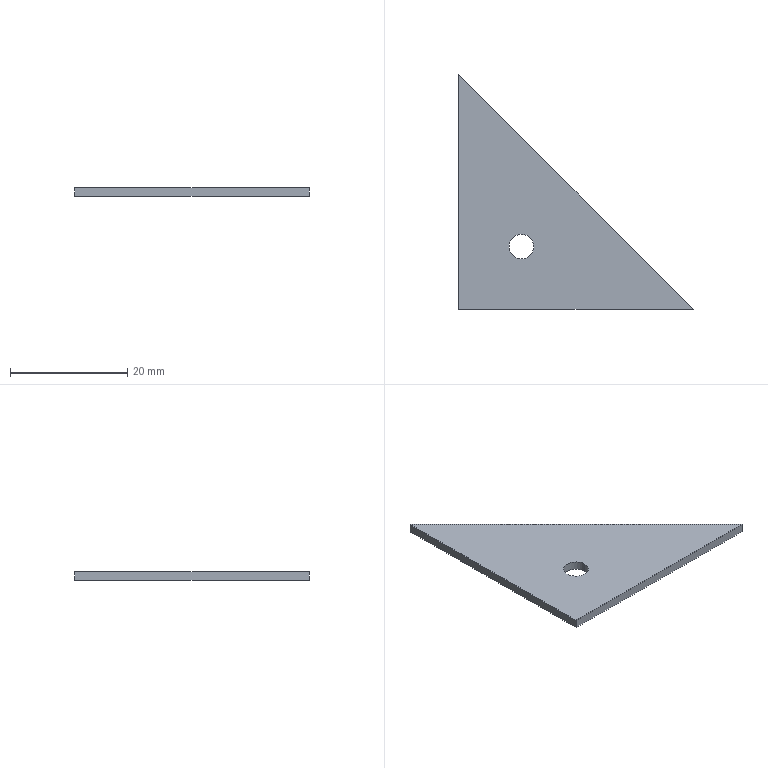Part | SolidWorks | features Cut 1, FlatPattern 1, SMBaseFlange 1, SheetMetal 1 | 1 solid | 7 faces | box 40 x 40 x 1.5 mm | volume 1179 mm3 | plane 5 | cylinder 2 | commonest cylinder face diameters 4.2 x2
STEP:
#1=CARTESIAN_POINT('',(7.968,10.858,-1.5));
#2=VERTEX_POINT('',#1);
#3=CARTESIAN_POINT('',(12.168,10.858,-1.5));
#4=VERTEX_POINT('',#3);
#5=CARTESIAN_POINT('',(10.068,10.858,-1.5));
#6=DIRECTION('',(0.,0.,1.));
#7=DIRECTION('',(1.,0.,0.));
#8=AXIS2_PLACEMENT_3D('',#5,#6,#7);
#9=CIRCLE('',#8,2.1);
#10=EDGE_CURVE('',#2,#4,#9,.T.);
#11=ORIENTED_EDGE('',*,*,#10,.F.);
#12=CARTESIAN_POINT('',(7.968,10.858,0.));
#13=VERTEX_POINT('',#12);
#14=CARTESIAN_POINT('',(7.968,10.858,-1.5));
#15=DIRECTION('',(0.,0.,1.));
#16=VECTOR('',#15,1000.);
#17=LINE('',#14,#16);
#18=EDGE_CURVE('',#2,#13,#17,.T.);
#19=ORIENTED_EDGE('',*,*,#18,.T.);
#20=CARTESIAN_POINT('',(12.168,10.858,0.));
#21=VERTEX_POINT('',#20);
#22=CARTESIAN_POINT('',(10.068,10.858,0.));
#23=DIRECTION('',(0.,0.,1.));
#24=DIRECTION('',(1.,0.,0.));
#25=AXIS2_PLACEMENT_3D('',#22,#23,#24);
#26=CIRCLE('',#25,2.1);
#27=EDGE_CURVE('',#13,#21,#26,.T.);
#28=ORIENTED_EDGE('',*,*,#27,.T.);
#29=CARTESIAN_POINT('',(12.168,10.858,-1.5));
#30=DIRECTION('',(0.,0.,1.));
#31=VECTOR('',#30,1000.);
#32=LINE('',#29,#31);
#33=EDGE_CURVE('',#4,#21,#32,.T.);
#34=ORIENTED_EDGE('',*,*,#33,.F.);
#35=EDGE_LOOP('',(#11,#19,#28,#34));
#36=FACE_OUTER_BOUND('',#35,.T.);
#37=CARTESIAN_POINT('',(10.068,10.858,-1.5));
#38=DIRECTION('',(0.,0.,1.));
#39=DIRECTION('',(1.,0.,0.));
#40=AXIS2_PLACEMENT_3D('',#37,#38,#39);
#41=CYLINDRICAL_SURFACE('',#40,2.1);
#42=ADVANCED_FACE('',(#36),#41,.F.);
#43=CARTESIAN_POINT('',(-0.6321,40.158,0.));
#44=VERTEX_POINT('',#43);
#45=CARTESIAN_POINT('',(-0.6321,0.158,0.));
#46=VERTEX_POINT('',#45);
#47=CARTESIAN_POINT('',(-0.6321,0.158,0.));
#48=DIRECTION('',(0.,-1.,0.));
#49=VECTOR('',#48,1000.);
#50=LINE('',#47,#49);
#51=EDGE_CURVE('',#44,#46,#50,.T.);
#52=ORIENTED_EDGE('',*,*,#51,.F.);
#53=CARTESIAN_POINT('',(-0.6321,40.158,-1.5));
#54=VERTEX_POINT('',#53);
#55=CARTESIAN_POINT('',(-0.6321,40.158,-1.5));
#56=DIRECTION('',(0.,0.,1.));
#57=VECTOR('',#56,1000.);
#58=LINE('',#55,#57);
#59=EDGE_CURVE('',#54,#44,#58,.T.);
#60=ORIENTED_EDGE('',*,*,#59,.F.);
#61=CARTESIAN_POINT('',(-0.6321,0.158,-1.5));
#62=VERTEX_POINT('',#61);
#63=CARTESIAN_POINT('',(-0.6321,0.158,-1.5));
#64=DIRECTION('',(0.,-1.,0.));
#65=VECTOR('',#64,1000.);
#66=LINE('',#63,#65);
#67=EDGE_CURVE('',#54,#62,#66,.T.);
#68=ORIENTED_EDGE('',*,*,#67,.T.);
#69=CARTESIAN_POINT('',(-0.6321,0.158,-1.5));
#70=DIRECTION('',(0.,0.,1.));
#71=VECTOR('',#70,1000.);
#72=LINE('',#69,#71);
#73=EDGE_CURVE('',#62,#46,#72,.T.);
#74=ORIENTED_EDGE('',*,*,#73,.T.);
#75=EDGE_LOOP('',(#52,#60,#68,#74));
#76=FACE_OUTER_BOUND('',#75,.T.);
#77=CARTESIAN_POINT('',(-0.6321,0.158,-1.5));
#78=DIRECTION('',(-1.,0.,0.));
#79=DIRECTION('',(0.,0.,1.));
#80=AXIS2_PLACEMENT_3D('',#77,#78,#79);
#81=PLANE('',#80);
#82=ADVANCED_FACE('',(#76),#81,.T.);
#83=CARTESIAN_POINT('',(39.368,0.158,0.));
#84=VERTEX_POINT('',#83);
#85=CARTESIAN_POINT('',(-0.6321,40.158,0.));
#86=DIRECTION('',(-0.7071,0.7071,0.));
#87=VECTOR('',#86,1000.);
#88=LINE('',#85,#87);
#89=EDGE_CURVE('',#84,#44,#88,.T.);
#90=ORIENTED_EDGE('',*,*,#89,.F.);
#91=CARTESIAN_POINT('',(39.368,0.158,-1.5));
#92=VERTEX_POINT('',#91);
#93=CARTESIAN_POINT('',(39.368,0.158,-1.5));
#94=DIRECTION('',(0.,0.,1.));
#95=VECTOR('',#94,1000.);
#96=LINE('',#93,#95);
#97=EDGE_CURVE('',#92,#84,#96,.T.);
#98=ORIENTED_EDGE('',*,*,#97,.F.);
#99=CARTESIAN_POINT('',(-0.6321,40.158,-1.5));
#100=DIRECTION('',(-0.7071,0.7071,0.));
#101=VECTOR('',#100,1000.);
#102=LINE('',#99,#101);
#103=EDGE_CURVE('',#92,#54,#102,.T.);
#104=ORIENTED_EDGE('',*,*,#103,.T.);
#105=ORIENTED_EDGE('',*,*,#59,.T.);
#106=EDGE_LOOP('',(#90,#98,#104,#105));
#107=FACE_OUTER_BOUND('',#106,.T.);
#108=CARTESIAN_POINT('',(-0.6321,40.158,-1.5));
#109=DIRECTION('',(0.7071,0.7071,0.));
#110=DIRECTION('',(-0.7071,0.7071,0.));
#111=AXIS2_PLACEMENT_3D('',#108,#109,#110);
#112=PLANE('',#111);
#113=ADVANCED_FACE('',(#107),#112,.T.);
#114=CARTESIAN_POINT('',(-0.6321,0.158,0.));
#115=DIRECTION('',(1.,0.,0.));
#116=VECTOR('',#115,1000.);
#117=LINE('',#114,#116);
#118=EDGE_CURVE('',#46,#84,#117,.T.);
#119=ORIENTED_EDGE('',*,*,#118,.F.);
#120=ORIENTED_EDGE('',*,*,#73,.F.);
#121=CARTESIAN_POINT('',(-0.6321,0.158,-1.5));
#122=DIRECTION('',(1.,0.,0.));
#123=VECTOR('',#122,1000.);
#124=LINE('',#121,#123);
#125=EDGE_CURVE('',#62,#92,#124,.T.);
#126=ORIENTED_EDGE('',*,*,#125,.T.);
#127=ORIENTED_EDGE('',*,*,#97,.T.);
#128=EDGE_LOOP('',(#119,#120,#126,#127));
#129=FACE_OUTER_BOUND('',#128,.T.);
#130=CARTESIAN_POINT('',(-0.6321,0.158,-1.5));
#131=DIRECTION('',(0.,-1.,0.));
#132=DIRECTION('',(0.,0.,-1.));
#133=AXIS2_PLACEMENT_3D('',#130,#131,#132);
#134=PLANE('',#133);
#135=ADVANCED_FACE('',(#129),#134,.T.);
#136=CARTESIAN_POINT('',(10.068,10.858,-1.5));
#137=DIRECTION('',(0.,0.,1.));
#138=DIRECTION('',(1.,0.,0.));
#139=AXIS2_PLACEMENT_3D('',#136,#137,#138);
#140=CIRCLE('',#139,2.1);
#141=EDGE_CURVE('',#4,#2,#140,.T.);
#142=ORIENTED_EDGE('',*,*,#141,.T.);
#143=ORIENTED_EDGE('',*,*,#10,.T.);
#144=EDGE_LOOP('',(#142,#143));
#145=FACE_BOUND('',#144,.T.);
#146=ORIENTED_EDGE('',*,*,#67,.F.);
#147=ORIENTED_EDGE('',*,*,#103,.F.);
#148=ORIENTED_EDGE('',*,*,#125,.F.);
#149=EDGE_LOOP('',(#146,#147,#148));
#150=FACE_OUTER_BOUND('',#149,.T.);
#151=CARTESIAN_POINT('',(0.,0.,-1.5));
#152=DIRECTION('',(0.,0.,-1.));
#153=DIRECTION('',(-1.,0.,0.));
#154=AXIS2_PLACEMENT_3D('',#151,#152,#153);
#155=PLANE('',#154);
#156=ADVANCED_FACE('',(#145,#150),#155,.T.);
#157=CARTESIAN_POINT('',(10.068,10.858,0.));
#158=DIRECTION('',(0.,0.,1.));
#159=DIRECTION('',(1.,0.,0.));
#160=AXIS2_PLACEMENT_3D('',#157,#158,#159);
#161=CIRCLE('',#160,2.1);
#162=EDGE_CURVE('',#21,#13,#161,.T.);
#163=ORIENTED_EDGE('',*,*,#162,.F.);
#164=ORIENTED_EDGE('',*,*,#27,.F.);
#165=EDGE_LOOP('',(#163,#164));
#166=FACE_BOUND('',#165,.T.);
#167=ORIENTED_EDGE('',*,*,#51,.T.);
#168=ORIENTED_EDGE('',*,*,#118,.T.);
#169=ORIENTED_EDGE('',*,*,#89,.T.);
#170=EDGE_LOOP('',(#167,#168,#169));
#171=FACE_OUTER_BOUND('',#170,.T.);
#172=CARTESIAN_POINT('',(0.,0.,0.));
#173=DIRECTION('',(0.,0.,-1.));
#174=DIRECTION('',(-1.,0.,0.));
#175=AXIS2_PLACEMENT_3D('',#172,#173,#174);
#176=PLANE('',#175);
#177=ADVANCED_FACE('',(#166,#171),#176,.F.);
#178=ORIENTED_EDGE('',*,*,#18,.F.);
#179=ORIENTED_EDGE('',*,*,#141,.F.);
#180=ORIENTED_EDGE('',*,*,#33,.T.);
#181=ORIENTED_EDGE('',*,*,#162,.T.);
#182=EDGE_LOOP('',(#178,#179,#180,#181));
#183=FACE_OUTER_BOUND('',#182,.T.);
#184=CARTESIAN_POINT('',(10.068,10.858,-1.5));
#185=DIRECTION('',(0.,0.,1.));
#186=DIRECTION('',(1.,0.,0.));
#187=AXIS2_PLACEMENT_3D('',#184,#185,#186);
#188=CYLINDRICAL_SURFACE('',#187,2.1);
#189=ADVANCED_FACE('',(#183),#188,.F.);
#190=CLOSED_SHELL('',(#42,#82,#113,#135,#156,#177,#189));
#191=MANIFOLD_SOLID_BREP('',#190);
#192=CARTESIAN_POINT('',(0.,0.,0.));
#193=DIRECTION('',(0.,0.,1.));
#194=DIRECTION('',(1.,0.,0.));
#195=AXIS2_PLACEMENT_3D('',#192,#193,#194);
#196=(LENGTH_UNIT()NAMED_UNIT(*)SI_UNIT(.MILLI.,.METRE.));
#197=UNCERTAINTY_MEASURE_WITH_UNIT(LENGTH_MEASURE(0.00001),#196,'','');
#198=(NAMED_UNIT(*)PLANE_ANGLE_UNIT()SI_UNIT($,.RADIAN.));
#199=(NAMED_UNIT(*)SI_UNIT($,.STERADIAN.)SOLID_ANGLE_UNIT());
#200=(GEOMETRIC_REPRESENTATION_CONTEXT(3)GLOBAL_UNCERTAINTY_ASSIGNED_CONTEXT((#197))GLOBAL_UNIT_ASSIGNED_CONTEXT((#196,#198,#199))REPRESENTATION_CONTEXT('',''));
#201=ADVANCED_BREP_SHAPE_REPRESENTATION('',(#191,#195),#200);